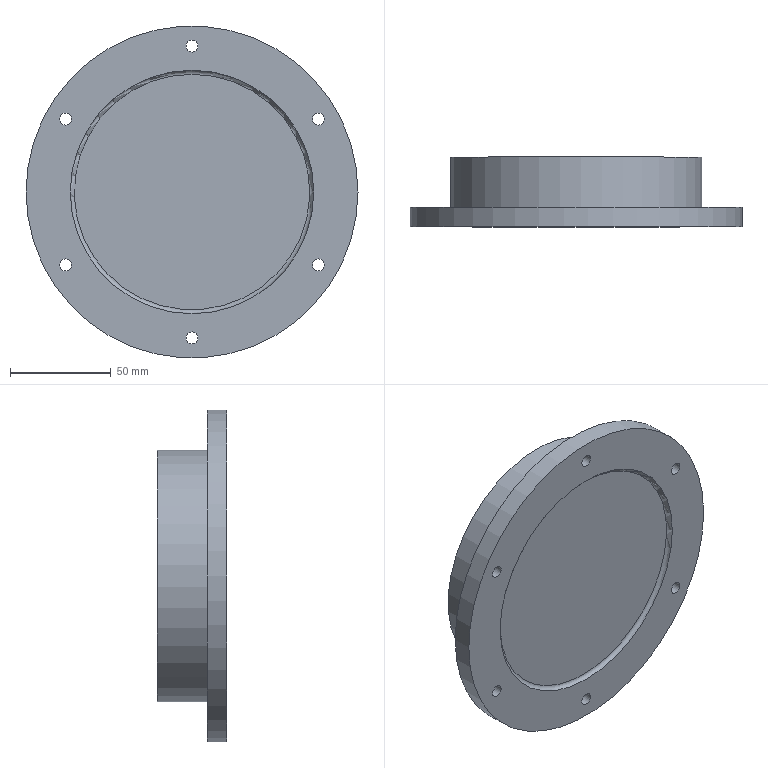Part | NX | features DATUM_CSYS 9, HOLE PACKAGE 9, SIMPLE HOLE 9, SKETCH 8, EXTRACT_DATUM_AXIS 6, EXTRACT_FACE 6, Instance Feature 5, BLEND 2, EXTRUDE 2, DELETE FACE 1, Pattern Feature 1 | 1 solid | 16 faces | box 165 x 34.6 x 165 mm | volume 267748 mm3 | cylinder 9 | plane 5 | torus 2 | commonest cylinder face diameters 6 x6 116 x1 125 x1 165 x1
STEP:
#1=CARTESIAN_POINT('',(82.5,0.,0.));
#2=VERTEX_POINT('',#1);
#3=CARTESIAN_POINT('',(0.,0.,0.));
#4=DIRECTION('',(0.,-1.,0.));
#5=DIRECTION('',(1.,0.,0.));
#6=AXIS2_PLACEMENT_3D('',#3,#4,#5);
#7=CIRCLE('',#6,82.5);
#8=EDGE_CURVE('',#2,#2,#7,.T.);
#9=ORIENTED_EDGE('',*,*,#8,.T.);
#10=EDGE_LOOP('',(#9));
#11=FACE_BOUND('',#10,.T.);
#12=CARTESIAN_POINT('',(82.5,-9.6,0.));
#13=VERTEX_POINT('',#12);
#14=CARTESIAN_POINT('',(0.,-9.6,0.));
#15=DIRECTION('',(0.,-1.,0.));
#16=DIRECTION('',(1.,0.,0.));
#17=AXIS2_PLACEMENT_3D('',#14,#15,#16);
#18=CIRCLE('',#17,82.5);
#19=EDGE_CURVE('',#13,#13,#18,.T.);
#20=ORIENTED_EDGE('',*,*,#19,.F.);
#21=EDGE_LOOP('',(#20));
#22=FACE_BOUND('',#21,.T.);
#23=CARTESIAN_POINT('',(0.,0.,0.));
#24=DIRECTION('',(0.,-1.,0.));
#25=DIRECTION('',(0.,0.,-1.));
#26=AXIS2_PLACEMENT_3D('',#23,#24,#25);
#27=CYLINDRICAL_SURFACE('',#26,82.5);
#28=ADVANCED_FACE('',(#11,#22),#27,.T.);
#29=CARTESIAN_POINT('',(-62.787,0.,33.25));
#30=VERTEX_POINT('',#29);
#31=CARTESIAN_POINT('',(-62.787,0.,36.25));
#32=DIRECTION('',(0.,-1.,0.));
#33=DIRECTION('',(0.,0.,-1.));
#34=AXIS2_PLACEMENT_3D('',#31,#32,#33);
#35=CIRCLE('',#34,3.);
#36=EDGE_CURVE('',#30,#30,#35,.T.);
#37=ORIENTED_EDGE('',*,*,#36,.T.);
#38=EDGE_LOOP('',(#37));
#39=FACE_BOUND('',#38,.T.);
#40=CARTESIAN_POINT('',(-62.787,0.,-39.25));
#41=VERTEX_POINT('',#40);
#42=CARTESIAN_POINT('',(-62.787,0.,-36.25));
#43=DIRECTION('',(0.,-1.,0.));
#44=DIRECTION('',(0.,0.,-1.));
#45=AXIS2_PLACEMENT_3D('',#42,#43,#44);
#46=CIRCLE('',#45,3.);
#47=EDGE_CURVE('',#41,#41,#46,.T.);
#48=ORIENTED_EDGE('',*,*,#47,.T.);
#49=EDGE_LOOP('',(#48));
#50=FACE_BOUND('',#49,.T.);
#51=CARTESIAN_POINT('',(0.,0.,-75.5));
#52=VERTEX_POINT('',#51);
#53=CARTESIAN_POINT('',(0.,0.,-72.5));
#54=DIRECTION('',(0.,-1.,0.));
#55=DIRECTION('',(0.,0.,-1.));
#56=AXIS2_PLACEMENT_3D('',#53,#54,#55);
#57=CIRCLE('',#56,3.);
#58=EDGE_CURVE('',#52,#52,#57,.T.);
#59=ORIENTED_EDGE('',*,*,#58,.T.);
#60=EDGE_LOOP('',(#59));
#61=FACE_BOUND('',#60,.T.);
#62=CARTESIAN_POINT('',(62.787,0.,-39.25));
#63=VERTEX_POINT('',#62);
#64=CARTESIAN_POINT('',(62.787,0.,-36.25));
#65=DIRECTION('',(0.,-1.,0.));
#66=DIRECTION('',(0.,0.,-1.));
#67=AXIS2_PLACEMENT_3D('',#64,#65,#66);
#68=CIRCLE('',#67,3.);
#69=EDGE_CURVE('',#63,#63,#68,.T.);
#70=ORIENTED_EDGE('',*,*,#69,.T.);
#71=EDGE_LOOP('',(#70));
#72=FACE_BOUND('',#71,.T.);
#73=CARTESIAN_POINT('',(62.787,0.,33.25));
#74=VERTEX_POINT('',#73);
#75=CARTESIAN_POINT('',(62.787,0.,36.25));
#76=DIRECTION('',(0.,-1.,0.));
#77=DIRECTION('',(0.,0.,-1.));
#78=AXIS2_PLACEMENT_3D('',#75,#76,#77);
#79=CIRCLE('',#78,3.);
#80=EDGE_CURVE('',#74,#74,#79,.T.);
#81=ORIENTED_EDGE('',*,*,#80,.T.);
#82=EDGE_LOOP('',(#81));
#83=FACE_BOUND('',#82,.T.);
#84=CARTESIAN_POINT('',(0.,0.,69.5));
#85=VERTEX_POINT('',#84);
#86=CARTESIAN_POINT('',(0.,0.,72.5));
#87=DIRECTION('',(0.,-1.,0.));
#88=DIRECTION('',(0.,0.,-1.));
#89=AXIS2_PLACEMENT_3D('',#86,#87,#88);
#90=CIRCLE('',#89,3.);
#91=EDGE_CURVE('',#85,#85,#90,.T.);
#92=ORIENTED_EDGE('',*,*,#91,.T.);
#93=EDGE_LOOP('',(#92));
#94=FACE_BOUND('',#93,.T.);
#95=CARTESIAN_POINT('',(62.5,0.,0.));
#96=VERTEX_POINT('',#95);
#97=CARTESIAN_POINT('',(0.,0.,0.));
#98=DIRECTION('',(0.,1.,0.));
#99=DIRECTION('',(1.,0.,0.));
#100=AXIS2_PLACEMENT_3D('',#97,#98,#99);
#101=CIRCLE('',#100,62.5);
#102=EDGE_CURVE('',#96,#96,#101,.T.);
#103=ORIENTED_EDGE('',*,*,#102,.F.);
#104=EDGE_LOOP('',(#103));
#105=FACE_BOUND('',#104,.T.);
#106=ORIENTED_EDGE('',*,*,#8,.F.);
#107=EDGE_LOOP('',(#106));
#108=FACE_BOUND('',#107,.T.);
#109=CARTESIAN_POINT('',(0.,0.,0.));
#110=DIRECTION('',(0.,-1.,0.));
#111=DIRECTION('',(0.,0.,-1.));
#112=AXIS2_PLACEMENT_3D('',#109,#110,#111);
#113=PLANE('',#112);
#114=ADVANCED_FACE('',(#39,#50,#61,#72,#83,#94,#105,#108),#113,.F.);
#115=CARTESIAN_POINT('',(-62.787,-9.6,39.25));
#116=VERTEX_POINT('',#115);
#117=CARTESIAN_POINT('',(-62.787,-9.6,36.25));
#118=DIRECTION('',(0.,1.,0.));
#119=DIRECTION('',(0.,0.,1.));
#120=AXIS2_PLACEMENT_3D('',#117,#118,#119);
#121=CIRCLE('',#120,3.);
#122=EDGE_CURVE('',#116,#116,#121,.T.);
#123=ORIENTED_EDGE('',*,*,#122,.T.);
#124=EDGE_LOOP('',(#123));
#125=FACE_BOUND('',#124,.T.);
#126=CARTESIAN_POINT('',(-62.787,-9.6,-33.25));
#127=VERTEX_POINT('',#126);
#128=CARTESIAN_POINT('',(-62.787,-9.6,-36.25));
#129=DIRECTION('',(0.,1.,0.));
#130=DIRECTION('',(0.,0.,1.));
#131=AXIS2_PLACEMENT_3D('',#128,#129,#130);
#132=CIRCLE('',#131,3.);
#133=EDGE_CURVE('',#127,#127,#132,.T.);
#134=ORIENTED_EDGE('',*,*,#133,.T.);
#135=EDGE_LOOP('',(#134));
#136=FACE_BOUND('',#135,.T.);
#137=CARTESIAN_POINT('',(0.,-9.6,-69.5));
#138=VERTEX_POINT('',#137);
#139=CARTESIAN_POINT('',(0.,-9.6,-72.5));
#140=DIRECTION('',(0.,1.,0.));
#141=DIRECTION('',(0.,0.,1.));
#142=AXIS2_PLACEMENT_3D('',#139,#140,#141);
#143=CIRCLE('',#142,3.);
#144=EDGE_CURVE('',#138,#138,#143,.T.);
#145=ORIENTED_EDGE('',*,*,#144,.T.);
#146=EDGE_LOOP('',(#145));
#147=FACE_BOUND('',#146,.T.);
#148=CARTESIAN_POINT('',(62.787,-9.6,-33.25));
#149=VERTEX_POINT('',#148);
#150=CARTESIAN_POINT('',(62.787,-9.6,-36.25));
#151=DIRECTION('',(0.,1.,0.));
#152=DIRECTION('',(0.,0.,1.));
#153=AXIS2_PLACEMENT_3D('',#150,#151,#152);
#154=CIRCLE('',#153,3.);
#155=EDGE_CURVE('',#149,#149,#154,.T.);
#156=ORIENTED_EDGE('',*,*,#155,.T.);
#157=EDGE_LOOP('',(#156));
#158=FACE_BOUND('',#157,.T.);
#159=CARTESIAN_POINT('',(62.787,-9.6,39.25));
#160=VERTEX_POINT('',#159);
#161=CARTESIAN_POINT('',(62.787,-9.6,36.25));
#162=DIRECTION('',(0.,1.,0.));
#163=DIRECTION('',(0.,0.,1.));
#164=AXIS2_PLACEMENT_3D('',#161,#162,#163);
#165=CIRCLE('',#164,3.);
#166=EDGE_CURVE('',#160,#160,#165,.T.);
#167=ORIENTED_EDGE('',*,*,#166,.T.);
#168=EDGE_LOOP('',(#167));
#169=FACE_BOUND('',#168,.T.);
#170=CARTESIAN_POINT('',(0.,-9.6,75.5));
#171=VERTEX_POINT('',#170);
#172=CARTESIAN_POINT('',(0.,-9.6,72.5));
#173=DIRECTION('',(0.,1.,0.));
#174=DIRECTION('',(0.,0.,1.));
#175=AXIS2_PLACEMENT_3D('',#172,#173,#174);
#176=CIRCLE('',#175,3.);
#177=EDGE_CURVE('',#171,#171,#176,.T.);
#178=ORIENTED_EDGE('',*,*,#177,.T.);
#179=EDGE_LOOP('',(#178));
#180=FACE_BOUND('',#179,.T.);
#181=CARTESIAN_POINT('',(0.,-9.6,60.5));
#182=VERTEX_POINT('',#181);
#183=CARTESIAN_POINT('',(0.,-9.6,0.));
#184=DIRECTION('',(0.,1.,0.));
#185=DIRECTION('',(0.,0.,1.));
#186=AXIS2_PLACEMENT_3D('',#183,#184,#185);
#187=CIRCLE('',#186,60.5);
#188=EDGE_CURVE('',#182,#182,#187,.T.);
#189=ORIENTED_EDGE('',*,*,#188,.T.);
#190=EDGE_LOOP('',(#189));
#191=FACE_BOUND('',#190,.T.);
#192=ORIENTED_EDGE('',*,*,#19,.T.);
#193=EDGE_LOOP('',(#192));
#194=FACE_BOUND('',#193,.T.);
#195=CARTESIAN_POINT('',(0.,-9.6,0.));
#196=DIRECTION('',(0.,-1.,0.));
#197=DIRECTION('',(0.,0.,-1.));
#198=AXIS2_PLACEMENT_3D('',#195,#196,#197);
#199=PLANE('',#198);
#200=ADVANCED_FACE('',(#125,#136,#147,#158,#169,#180,#191,#194),#199,.T.);
#201=ORIENTED_EDGE('',*,*,#102,.T.);
#202=EDGE_LOOP('',(#201));
#203=FACE_BOUND('',#202,.T.);
#204=CARTESIAN_POINT('',(62.5,25.,0.));
#205=VERTEX_POINT('',#204);
#206=CARTESIAN_POINT('',(0.,25.,0.));
#207=DIRECTION('',(0.,1.,0.));
#208=DIRECTION('',(1.,0.,0.));
#209=AXIS2_PLACEMENT_3D('',#206,#207,#208);
#210=CIRCLE('',#209,62.5);
#211=EDGE_CURVE('',#205,#205,#210,.T.);
#212=ORIENTED_EDGE('',*,*,#211,.F.);
#213=EDGE_LOOP('',(#212));
#214=FACE_BOUND('',#213,.T.);
#215=CARTESIAN_POINT('',(0.,0.,0.));
#216=DIRECTION('',(0.,1.,0.));
#217=DIRECTION('',(0.,0.,1.));
#218=AXIS2_PLACEMENT_3D('',#215,#216,#217);
#219=CYLINDRICAL_SURFACE('',#218,62.5);
#220=ADVANCED_FACE('',(#203,#214),#219,.T.);
#221=CARTESIAN_POINT('',(0.,25.,-58.));
#222=VERTEX_POINT('',#221);
#223=CARTESIAN_POINT('',(0.,25.,0.));
#224=DIRECTION('',(0.,-1.,0.));
#225=DIRECTION('',(0.,0.,-1.));
#226=AXIS2_PLACEMENT_3D('',#223,#224,#225);
#227=CIRCLE('',#226,58.);
#228=EDGE_CURVE('',#222,#222,#227,.T.);
#229=ORIENTED_EDGE('',*,*,#228,.T.);
#230=EDGE_LOOP('',(#229));
#231=FACE_BOUND('',#230,.T.);
#232=ORIENTED_EDGE('',*,*,#211,.T.);
#233=EDGE_LOOP('',(#232));
#234=FACE_BOUND('',#233,.T.);
#235=CARTESIAN_POINT('',(0.,25.,0.));
#236=DIRECTION('',(0.,1.,0.));
#237=DIRECTION('',(0.,0.,1.));
#238=AXIS2_PLACEMENT_3D('',#235,#236,#237);
#239=PLANE('',#238);
#240=ADVANCED_FACE('',(#231,#234),#239,.T.);
#241=CARTESIAN_POINT('',(0.,4.,-53.));
#242=VERTEX_POINT('',#241);
#243=CARTESIAN_POINT('',(0.,4.,0.));
#244=DIRECTION('',(0.,-1.,0.));
#245=DIRECTION('',(0.,0.,-1.));
#246=AXIS2_PLACEMENT_3D('',#243,#244,#245);
#247=CIRCLE('',#246,53.);
#248=EDGE_CURVE('',#242,#242,#247,.F.);
#249=ORIENTED_EDGE('',*,*,#248,.T.);
#250=EDGE_LOOP('',(#249));
#251=FACE_BOUND('',#250,.T.);
#252=CARTESIAN_POINT('',(0.,4.,0.));
#253=DIRECTION('',(0.,-1.,0.));
#254=DIRECTION('',(0.,0.,-1.));
#255=AXIS2_PLACEMENT_3D('',#252,#253,#254);
#256=PLANE('',#255);
#257=ADVANCED_FACE('',(#251),#256,.F.);
#258=CARTESIAN_POINT('',(0.,9.,-58.));
#259=VERTEX_POINT('',#258);
#260=CARTESIAN_POINT('',(0.,9.,0.));
#261=DIRECTION('',(0.,-1.,0.));
#262=DIRECTION('',(0.,0.,-1.));
#263=AXIS2_PLACEMENT_3D('',#260,#261,#262);
#264=CIRCLE('',#263,58.);
#265=EDGE_CURVE('',#259,#259,#264,.T.);
#266=ORIENTED_EDGE('',*,*,#265,.T.);
#267=EDGE_LOOP('',(#266));
#268=FACE_BOUND('',#267,.T.);
#269=ORIENTED_EDGE('',*,*,#228,.F.);
#270=EDGE_LOOP('',(#269));
#271=FACE_BOUND('',#270,.T.);
#272=CARTESIAN_POINT('',(0.,25.,0.));
#273=DIRECTION('',(0.,-1.,0.));
#274=DIRECTION('',(0.,0.,-1.));
#275=AXIS2_PLACEMENT_3D('',#272,#273,#274);
#276=CYLINDRICAL_SURFACE('',#275,58.);
#277=ADVANCED_FACE('',(#268,#271),#276,.F.);
#278=CARTESIAN_POINT('',(0.,-7.6,58.5));
#279=VERTEX_POINT('',#278);
#280=CARTESIAN_POINT('',(0.,-7.6,0.));
#281=DIRECTION('',(0.,1.,0.));
#282=DIRECTION('',(0.,0.,1.));
#283=AXIS2_PLACEMENT_3D('',#280,#281,#282);
#284=CIRCLE('',#283,58.5);
#285=EDGE_CURVE('',#279,#279,#284,.F.);
#286=ORIENTED_EDGE('',*,*,#285,.T.);
#287=EDGE_LOOP('',(#286));
#288=FACE_BOUND('',#287,.T.);
#289=CARTESIAN_POINT('',(0.,-7.6,0.));
#290=DIRECTION('',(0.,1.,0.));
#291=DIRECTION('',(0.,0.,1.));
#292=AXIS2_PLACEMENT_3D('',#289,#290,#291);
#293=PLANE('',#292);
#294=ADVANCED_FACE('',(#288),#293,.F.);
#295=ORIENTED_EDGE('',*,*,#188,.F.);
#296=EDGE_LOOP('',(#295));
#297=FACE_BOUND('',#296,.T.);
#298=ORIENTED_EDGE('',*,*,#285,.F.);
#299=EDGE_LOOP('',(#298));
#300=FACE_BOUND('',#299,.T.);
#301=CARTESIAN_POINT('',(0.,-9.6,0.));
#302=DIRECTION('',(0.,1.,0.));
#303=DIRECTION('',(0.,0.,1.));
#304=AXIS2_PLACEMENT_3D('',#301,#302,#303);
#305=TOROIDAL_SURFACE('',#304,58.5,2.);
#306=ADVANCED_FACE('',(#297,#300),#305,.F.);
#307=ORIENTED_EDGE('',*,*,#265,.F.);
#308=EDGE_LOOP('',(#307));
#309=FACE_BOUND('',#308,.T.);
#310=ORIENTED_EDGE('',*,*,#248,.F.);
#311=EDGE_LOOP('',(#310));
#312=FACE_BOUND('',#311,.T.);
#313=CARTESIAN_POINT('',(0.,9.,0.));
#314=DIRECTION('',(0.,-1.,0.));
#315=DIRECTION('',(0.,0.,-1.));
#316=AXIS2_PLACEMENT_3D('',#313,#314,#315);
#317=TOROIDAL_SURFACE('',#316,53.,5.);
#318=ADVANCED_FACE('',(#309,#312),#317,.F.);
#319=ORIENTED_EDGE('',*,*,#177,.F.);
#320=EDGE_LOOP('',(#319));
#321=FACE_BOUND('',#320,.T.);
#322=ORIENTED_EDGE('',*,*,#91,.F.);
#323=EDGE_LOOP('',(#322));
#324=FACE_BOUND('',#323,.T.);
#325=CARTESIAN_POINT('',(0.,-9.6,72.5));
#326=DIRECTION('',(0.,1.,0.));
#327=DIRECTION('',(0.,0.,1.));
#328=AXIS2_PLACEMENT_3D('',#325,#326,#327);
#329=CYLINDRICAL_SURFACE('',#328,3.);
#330=ADVANCED_FACE('',(#321,#324),#329,.F.);
#331=ORIENTED_EDGE('',*,*,#166,.F.);
#332=EDGE_LOOP('',(#331));
#333=FACE_BOUND('',#332,.T.);
#334=ORIENTED_EDGE('',*,*,#80,.F.);
#335=EDGE_LOOP('',(#334));
#336=FACE_BOUND('',#335,.T.);
#337=CARTESIAN_POINT('',(62.787,-9.6,36.25));
#338=DIRECTION('',(0.,1.,0.));
#339=DIRECTION('',(0.,0.,1.));
#340=AXIS2_PLACEMENT_3D('',#337,#338,#339);
#341=CYLINDRICAL_SURFACE('',#340,3.);
#342=ADVANCED_FACE('',(#333,#336),#341,.F.);
#343=ORIENTED_EDGE('',*,*,#155,.F.);
#344=EDGE_LOOP('',(#343));
#345=FACE_BOUND('',#344,.T.);
#346=ORIENTED_EDGE('',*,*,#69,.F.);
#347=EDGE_LOOP('',(#346));
#348=FACE_BOUND('',#347,.T.);
#349=CARTESIAN_POINT('',(62.787,-9.6,-36.25));
#350=DIRECTION('',(0.,1.,0.));
#351=DIRECTION('',(0.,0.,1.));
#352=AXIS2_PLACEMENT_3D('',#349,#350,#351);
#353=CYLINDRICAL_SURFACE('',#352,3.);
#354=ADVANCED_FACE('',(#345,#348),#353,.F.);
#355=ORIENTED_EDGE('',*,*,#144,.F.);
#356=EDGE_LOOP('',(#355));
#357=FACE_BOUND('',#356,.T.);
#358=ORIENTED_EDGE('',*,*,#58,.F.);
#359=EDGE_LOOP('',(#358));
#360=FACE_BOUND('',#359,.T.);
#361=CARTESIAN_POINT('',(0.,-9.6,-72.5));
#362=DIRECTION('',(0.,1.,0.));
#363=DIRECTION('',(0.,0.,1.));
#364=AXIS2_PLACEMENT_3D('',#361,#362,#363);
#365=CYLINDRICAL_SURFACE('',#364,3.);
#366=ADVANCED_FACE('',(#357,#360),#365,.F.);
#367=ORIENTED_EDGE('',*,*,#133,.F.);
#368=EDGE_LOOP('',(#367));
#369=FACE_BOUND('',#368,.T.);
#370=ORIENTED_EDGE('',*,*,#47,.F.);
#371=EDGE_LOOP('',(#370));
#372=FACE_BOUND('',#371,.T.);
#373=CARTESIAN_POINT('',(-62.787,-9.6,-36.25));
#374=DIRECTION('',(0.,1.,0.));
#375=DIRECTION('',(0.,0.,1.));
#376=AXIS2_PLACEMENT_3D('',#373,#374,#375);
#377=CYLINDRICAL_SURFACE('',#376,3.);
#378=ADVANCED_FACE('',(#369,#372),#377,.F.);
#379=ORIENTED_EDGE('',*,*,#122,.F.);
#380=EDGE_LOOP('',(#379));
#381=FACE_BOUND('',#380,.T.);
#382=ORIENTED_EDGE('',*,*,#36,.F.);
#383=EDGE_LOOP('',(#382));
#384=FACE_BOUND('',#383,.T.);
#385=CARTESIAN_POINT('',(-62.787,-9.6,36.25));
#386=DIRECTION('',(0.,1.,0.));
#387=DIRECTION('',(0.,0.,1.));
#388=AXIS2_PLACEMENT_3D('',#385,#386,#387);
#389=CYLINDRICAL_SURFACE('',#388,3.);
#390=ADVANCED_FACE('',(#381,#384),#389,.F.);
#391=CLOSED_SHELL('',(#28,#114,#200,#220,#240,#257,#277,#294,#306,#318,#330,#342,#354,#366,#378,#390));
#392=MANIFOLD_SOLID_BREP('',#391);
#393=(LENGTH_UNIT()NAMED_UNIT(*)SI_UNIT(.MILLI.,.METRE.));
#394=UNCERTAINTY_MEASURE_WITH_UNIT(LENGTH_MEASURE(0.00001),#393,'','');
#395=(NAMED_UNIT(*)PLANE_ANGLE_UNIT()SI_UNIT($,.RADIAN.));
#396=(NAMED_UNIT(*)SI_UNIT($,.STERADIAN.)SOLID_ANGLE_UNIT());
#397=(GEOMETRIC_REPRESENTATION_CONTEXT(3)GLOBAL_UNCERTAINTY_ASSIGNED_CONTEXT((#394))GLOBAL_UNIT_ASSIGNED_CONTEXT((#393,#395,#396))REPRESENTATION_CONTEXT('',''));
#398=ADVANCED_BREP_SHAPE_REPRESENTATION('',(#392),#397);